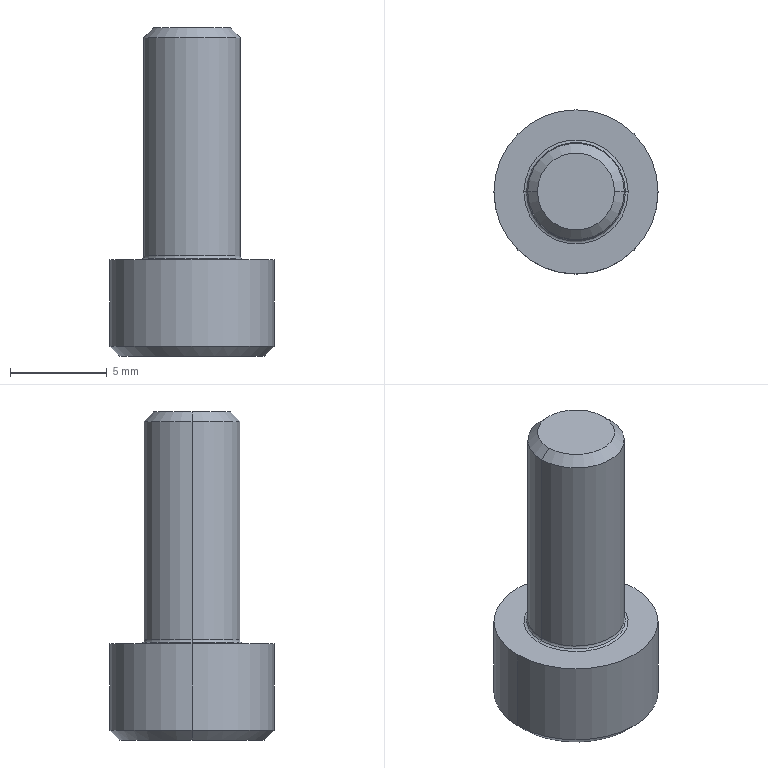Part | Creo | 1 solid | 23 faces | box 8.5 x 8.5 x 17 mm | volume 472.559 mm3 | plane 9 | cone 6 | cylinder 4 | torus 4 | commonest cylinder face diameters 5 x2 8.5 x2
STEP:
#1=CARTESIAN_POINT('',(-86.191,-52.429,-197.5));
#2=VERTEX_POINT('',#1);
#3=CARTESIAN_POINT('',(-87.345,-54.429,-197.5));
#4=VERTEX_POINT('',#3);
#5=CARTESIAN_POINT('',(-86.191,-52.429,-197.5));
#6=CARTESIAN_POINT('',(-86.244,-52.522,-197.469));
#7=CARTESIAN_POINT('',(-86.352,-52.708,-197.413));
#8=CARTESIAN_POINT('',(-86.517,-52.995,-197.352));
#9=CARTESIAN_POINT('',(-86.684,-53.284,-197.32));
#10=CARTESIAN_POINT('',(-86.851,-53.573,-197.32));
#11=CARTESIAN_POINT('',(-87.018,-53.862,-197.352));
#12=CARTESIAN_POINT('',(-87.183,-54.149,-197.413));
#13=CARTESIAN_POINT('',(-87.292,-54.336,-197.469));
#14=CARTESIAN_POINT('',(-87.345,-54.429,-197.5));
#15=B_SPLINE_CURVE_WITH_KNOTS('',3,(#5,#6,#7,#8,#9,#10,#11,#12,#13,#14),.UNSPECIFIED.,.F.,.F.,(4,1,1,1,1,1,1,4),(0.,0.1429,0.2857,0.4286,0.5714,0.7143,0.8571,1.),.UNSPECIFIED.);
#16=EDGE_CURVE('',#2,#4,#15,.T.);
#17=ORIENTED_EDGE('',*,*,#16,.F.);
#18=CARTESIAN_POINT('',(-88.5,-52.429,-196.167));
#19=VERTEX_POINT('',#18);
#20=CARTESIAN_POINT('',(-88.5,-52.429,-196.167));
#21=DIRECTION('',(0.866,0.,-0.5));
#22=VECTOR('',#21,2.667);
#23=LINE('',#20,#22);
#24=EDGE_CURVE('',#19,#2,#23,.T.);
#25=ORIENTED_EDGE('',*,*,#24,.F.);
#26=CARTESIAN_POINT('',(-90.809,-52.429,-197.5));
#27=VERTEX_POINT('',#26);
#28=CARTESIAN_POINT('',(-88.5,-52.429,-196.167));
#29=DIRECTION('',(-0.866,0.,-0.5));
#30=VECTOR('',#29,2.667);
#31=LINE('',#28,#30);
#32=EDGE_CURVE('',#19,#27,#31,.T.);
#33=ORIENTED_EDGE('',*,*,#32,.T.);
#34=CARTESIAN_POINT('',(-89.655,-54.429,-197.5));
#35=VERTEX_POINT('',#34);
#36=CARTESIAN_POINT('',(-89.655,-54.429,-197.5));
#37=CARTESIAN_POINT('',(-89.708,-54.336,-197.469));
#38=CARTESIAN_POINT('',(-89.817,-54.149,-197.413));
#39=CARTESIAN_POINT('',(-89.982,-53.862,-197.352));
#40=CARTESIAN_POINT('',(-90.149,-53.573,-197.32));
#41=CARTESIAN_POINT('',(-90.316,-53.284,-197.32));
#42=CARTESIAN_POINT('',(-90.483,-52.995,-197.352));
#43=CARTESIAN_POINT('',(-90.648,-52.708,-197.413));
#44=CARTESIAN_POINT('',(-90.756,-52.522,-197.469));
#45=CARTESIAN_POINT('',(-90.809,-52.429,-197.5));
#46=B_SPLINE_CURVE_WITH_KNOTS('',3,(#36,#37,#38,#39,#40,#41,#42,#43,#44,#45),.UNSPECIFIED.,.F.,.F.,(4,1,1,1,1,1,1,4),(0.,0.1429,0.2857,0.4286,0.5714,0.7143,0.8571,1.),.UNSPECIFIED.);
#47=EDGE_CURVE('',#35,#27,#46,.T.);
#48=ORIENTED_EDGE('',*,*,#47,.F.);
#49=CARTESIAN_POINT('',(-87.345,-54.429,-197.5));
#50=CARTESIAN_POINT('',(-87.453,-54.429,-197.469));
#51=CARTESIAN_POINT('',(-87.669,-54.429,-197.413));
#52=CARTESIAN_POINT('',(-88.,-54.429,-197.352));
#53=CARTESIAN_POINT('',(-88.334,-54.429,-197.32));
#54=CARTESIAN_POINT('',(-88.668,-54.429,-197.32));
#55=CARTESIAN_POINT('',(-89.002,-54.429,-197.352));
#56=CARTESIAN_POINT('',(-89.332,-54.429,-197.413));
#57=CARTESIAN_POINT('',(-89.548,-54.429,-197.469));
#58=CARTESIAN_POINT('',(-89.655,-54.429,-197.5));
#59=B_SPLINE_CURVE_WITH_KNOTS('',3,(#49,#50,#51,#52,#53,#54,#55,#56,#57,#58),.UNSPECIFIED.,.F.,.F.,(4,1,1,1,1,1,1,4),(0.,0.1429,0.2857,0.4286,0.5714,0.7143,0.8571,1.),.UNSPECIFIED.);
#60=EDGE_CURVE('',#4,#35,#59,.T.);
#61=ORIENTED_EDGE('',*,*,#60,.F.);
#62=EDGE_LOOP('',(#17,#25,#33,#48,#61));
#63=FACE_OUTER_BOUND('',#62,.F.);
#64=CARTESIAN_POINT('',(-88.5,-52.429,-196.847));
#65=DIRECTION('',(0.,0.,-1.));
#66=DIRECTION('',(1.,0.,0.));
#67=AXIS2_PLACEMENT_3D('',#64,#65,#66);
#68=CONICAL_SURFACE('',#67,1.178,60.);
#69=ADVANCED_FACE('',(#63),#68,.F.);
#70=CARTESIAN_POINT('',(-87.345,-54.429,-200.));
#71=VERTEX_POINT('',#70);
#72=CARTESIAN_POINT('',(-86.191,-52.429,-200.));
#73=VERTEX_POINT('',#72);
#74=CARTESIAN_POINT('',(-87.345,-54.429,-200.));
#75=DIRECTION('',(0.5,0.866,0.));
#76=VECTOR('',#75,2.309);
#77=LINE('',#74,#76);
#78=EDGE_CURVE('',#71,#73,#77,.T.);
#79=ORIENTED_EDGE('',*,*,#78,.T.);
#80=CARTESIAN_POINT('',(-86.191,-52.429,-197.5));
#81=DIRECTION('',(0.,0.,-1.));
#82=VECTOR('',#81,2.5);
#83=LINE('',#80,#82);
#84=EDGE_CURVE('',#2,#73,#83,.T.);
#85=ORIENTED_EDGE('',*,*,#84,.F.);
#86=ORIENTED_EDGE('',*,*,#16,.T.);
#87=CARTESIAN_POINT('',(-87.345,-54.429,-197.5));
#88=DIRECTION('',(0.,0.,-1.));
#89=VECTOR('',#88,2.5);
#90=LINE('',#87,#89);
#91=EDGE_CURVE('',#4,#71,#90,.T.);
#92=ORIENTED_EDGE('',*,*,#91,.T.);
#93=EDGE_LOOP('',(#79,#85,#86,#92));
#94=FACE_OUTER_BOUND('',#93,.F.);
#95=CARTESIAN_POINT('',(-87.345,-54.429,-197.5));
#96=DIRECTION('',(-0.866,0.5,0.));
#97=DIRECTION('',(-0.5,-0.866,0.));
#98=AXIS2_PLACEMENT_3D('',#95,#96,#97);
#99=PLANE('',#98);
#100=ADVANCED_FACE('',(#94),#99,.T.);
#101=CARTESIAN_POINT('',(-92.25,-52.429,-200.));
#102=VERTEX_POINT('',#101);
#103=CARTESIAN_POINT('',(-84.75,-52.429,-200.));
#104=VERTEX_POINT('',#103);
#105=CARTESIAN_POINT('',(-88.5,-52.429,-200.));
#106=DIRECTION('',(0.,0.,-1.));
#107=DIRECTION('',(-1.,0.,0.));
#108=AXIS2_PLACEMENT_3D('',#105,#106,#107);
#109=CIRCLE('',#108,3.75);
#110=EDGE_CURVE('',#102,#104,#109,.T.);
#111=ORIENTED_EDGE('',*,*,#110,.F.);
#112=CARTESIAN_POINT('',(-88.5,-52.429,-200.));
#113=DIRECTION('',(0.,0.,-1.));
#114=DIRECTION('',(1.,0.,0.));
#115=AXIS2_PLACEMENT_3D('',#112,#113,#114);
#116=CIRCLE('',#115,3.75);
#117=EDGE_CURVE('',#104,#102,#116,.T.);
#118=ORIENTED_EDGE('',*,*,#117,.F.);
#119=EDGE_LOOP('',(#111,#118));
#120=FACE_OUTER_BOUND('',#119,.F.);
#121=CARTESIAN_POINT('',(-90.809,-52.429,-200.));
#122=VERTEX_POINT('',#121);
#123=CARTESIAN_POINT('',(-89.655,-54.429,-200.));
#124=VERTEX_POINT('',#123);
#125=CARTESIAN_POINT('',(-90.809,-52.429,-200.));
#126=DIRECTION('',(0.5,-0.866,0.));
#127=VECTOR('',#126,2.309);
#128=LINE('',#125,#127);
#129=EDGE_CURVE('',#122,#124,#128,.T.);
#130=ORIENTED_EDGE('',*,*,#129,.F.);
#131=CARTESIAN_POINT('',(-89.655,-50.429,-200.));
#132=VERTEX_POINT('',#131);
#133=CARTESIAN_POINT('',(-89.655,-50.429,-200.));
#134=DIRECTION('',(-0.5,-0.866,0.));
#135=VECTOR('',#134,2.309);
#136=LINE('',#133,#135);
#137=EDGE_CURVE('',#132,#122,#136,.T.);
#138=ORIENTED_EDGE('',*,*,#137,.F.);
#139=CARTESIAN_POINT('',(-87.345,-50.429,-200.));
#140=VERTEX_POINT('',#139);
#141=CARTESIAN_POINT('',(-89.655,-50.429,-200.));
#142=DIRECTION('',(1.,0.,0.));
#143=VECTOR('',#142,2.309);
#144=LINE('',#141,#143);
#145=EDGE_CURVE('',#132,#140,#144,.T.);
#146=ORIENTED_EDGE('',*,*,#145,.T.);
#147=CARTESIAN_POINT('',(-86.191,-52.429,-200.));
#148=DIRECTION('',(-0.5,0.866,0.));
#149=VECTOR('',#148,2.309);
#150=LINE('',#147,#149);
#151=EDGE_CURVE('',#73,#140,#150,.T.);
#152=ORIENTED_EDGE('',*,*,#151,.F.);
#153=ORIENTED_EDGE('',*,*,#78,.F.);
#154=CARTESIAN_POINT('',(-87.345,-54.429,-200.));
#155=DIRECTION('',(-1.,0.,0.));
#156=VECTOR('',#155,2.309);
#157=LINE('',#154,#156);
#158=EDGE_CURVE('',#71,#124,#157,.T.);
#159=ORIENTED_EDGE('',*,*,#158,.T.);
#160=EDGE_LOOP('',(#130,#138,#146,#152,#153,#159));
#161=FACE_BOUND('',#160,.F.);
#162=CARTESIAN_POINT('',(-88.5,-52.429,-200.));
#163=DIRECTION('',(0.,0.,-1.));
#164=DIRECTION('',(1.,0.,0.));
#165=AXIS2_PLACEMENT_3D('',#162,#163,#164);
#166=PLANE('',#165);
#167=ADVANCED_FACE('',(#120,#161),#166,.T.);
#168=CARTESIAN_POINT('',(-92.75,-52.429,-199.5));
#169=VERTEX_POINT('',#168);
#170=CARTESIAN_POINT('',(-84.25,-52.429,-199.5));
#171=VERTEX_POINT('',#170);
#172=CARTESIAN_POINT('',(-88.5,-52.429,-199.5));
#173=DIRECTION('',(0.,0.,-1.));
#174=DIRECTION('',(-1.,0.,0.));
#175=AXIS2_PLACEMENT_3D('',#172,#173,#174);
#176=CIRCLE('',#175,4.25);
#177=EDGE_CURVE('',#169,#171,#176,.T.);
#178=ORIENTED_EDGE('',*,*,#177,.F.);
#179=CARTESIAN_POINT('',(-92.25,-52.429,-200.));
#180=DIRECTION('',(-0.7071,0.,0.7071));
#181=VECTOR('',#180,0.7071);
#182=LINE('',#179,#181);
#183=EDGE_CURVE('',#102,#169,#182,.T.);
#184=ORIENTED_EDGE('',*,*,#183,.F.);
#185=ORIENTED_EDGE('',*,*,#110,.T.);
#186=CARTESIAN_POINT('',(-84.75,-52.429,-200.));
#187=DIRECTION('',(0.7071,0.,0.7071));
#188=VECTOR('',#187,0.7071);
#189=LINE('',#186,#188);
#190=EDGE_CURVE('',#104,#171,#189,.T.);
#191=ORIENTED_EDGE('',*,*,#190,.T.);
#192=EDGE_LOOP('',(#178,#184,#185,#191));
#193=FACE_OUTER_BOUND('',#192,.F.);
#194=CARTESIAN_POINT('',(-88.5,-52.429,-199.75));
#195=DIRECTION('',(0.,0.,1.));
#196=DIRECTION('',(-1.,0.,0.));
#197=AXIS2_PLACEMENT_3D('',#194,#195,#196);
#198=CONICAL_SURFACE('',#197,4.,45.);
#199=ADVANCED_FACE('',(#193),#198,.T.);
#200=ORIENTED_EDGE('',*,*,#177,.T.);
#201=CARTESIAN_POINT('',(-84.25,-52.429,-195.));
#202=VERTEX_POINT('',#201);
#203=CARTESIAN_POINT('',(-84.25,-52.429,-195.));
#204=DIRECTION('',(0.,0.,-1.));
#205=VECTOR('',#204,4.5);
#206=LINE('',#203,#205);
#207=EDGE_CURVE('',#202,#171,#206,.T.);
#208=ORIENTED_EDGE('',*,*,#207,.F.);
#209=CARTESIAN_POINT('',(-92.75,-52.429,-195.));
#210=VERTEX_POINT('',#209);
#211=CARTESIAN_POINT('',(-88.5,-52.429,-195.));
#212=DIRECTION('',(0.,0.,1.));
#213=DIRECTION('',(1.,0.,0.));
#214=AXIS2_PLACEMENT_3D('',#211,#212,#213);
#215=CIRCLE('',#214,4.25);
#216=EDGE_CURVE('',#202,#210,#215,.T.);
#217=ORIENTED_EDGE('',*,*,#216,.T.);
#218=CARTESIAN_POINT('',(-92.75,-52.429,-195.));
#219=DIRECTION('',(0.,0.,-1.));
#220=VECTOR('',#219,4.5);
#221=LINE('',#218,#220);
#222=EDGE_CURVE('',#210,#169,#221,.T.);
#223=ORIENTED_EDGE('',*,*,#222,.T.);
#224=EDGE_LOOP('',(#200,#208,#217,#223));
#225=FACE_OUTER_BOUND('',#224,.F.);
#226=CARTESIAN_POINT('',(-88.5,-52.429,-195.));
#227=DIRECTION('',(0.,0.,-1.));
#228=DIRECTION('',(1.,0.,0.));
#229=AXIS2_PLACEMENT_3D('',#226,#227,#228);
#230=CYLINDRICAL_SURFACE('',#229,4.25);
#231=ADVANCED_FACE('',(#225),#230,.T.);
#232=CARTESIAN_POINT('',(-88.5,-52.429,-199.5));
#233=DIRECTION('',(0.,0.,-1.));
#234=DIRECTION('',(1.,0.,0.));
#235=AXIS2_PLACEMENT_3D('',#232,#233,#234);
#236=CIRCLE('',#235,4.25);
#237=EDGE_CURVE('',#171,#169,#236,.T.);
#238=ORIENTED_EDGE('',*,*,#237,.T.);
#239=ORIENTED_EDGE('',*,*,#222,.F.);
#240=CARTESIAN_POINT('',(-88.5,-52.429,-195.));
#241=DIRECTION('',(0.,0.,1.));
#242=DIRECTION('',(-1.,0.,0.));
#243=AXIS2_PLACEMENT_3D('',#240,#241,#242);
#244=CIRCLE('',#243,4.25);
#245=EDGE_CURVE('',#210,#202,#244,.T.);
#246=ORIENTED_EDGE('',*,*,#245,.T.);
#247=ORIENTED_EDGE('',*,*,#207,.T.);
#248=EDGE_LOOP('',(#238,#239,#246,#247));
#249=FACE_OUTER_BOUND('',#248,.F.);
#250=CARTESIAN_POINT('',(-88.5,-52.429,-195.));
#251=DIRECTION('',(0.,0.,-1.));
#252=DIRECTION('',(1.,0.,0.));
#253=AXIS2_PLACEMENT_3D('',#250,#251,#252);
#254=CYLINDRICAL_SURFACE('',#253,4.25);
#255=ADVANCED_FACE('',(#249),#254,.T.);
#256=ORIENTED_EDGE('',*,*,#237,.F.);
#257=ORIENTED_EDGE('',*,*,#190,.F.);
#258=ORIENTED_EDGE('',*,*,#117,.T.);
#259=ORIENTED_EDGE('',*,*,#183,.T.);
#260=EDGE_LOOP('',(#256,#257,#258,#259));
#261=FACE_OUTER_BOUND('',#260,.F.);
#262=CARTESIAN_POINT('',(-88.5,-52.429,-199.75));
#263=DIRECTION('',(0.,0.,1.));
#264=DIRECTION('',(-1.,0.,0.));
#265=AXIS2_PLACEMENT_3D('',#262,#263,#264);
#266=CONICAL_SURFACE('',#265,4.,45.);
#267=ADVANCED_FACE('',(#261),#266,.T.);
#268=ORIENTED_EDGE('',*,*,#245,.F.);
#269=ORIENTED_EDGE('',*,*,#216,.F.);
#270=EDGE_LOOP('',(#268,#269));
#271=FACE_OUTER_BOUND('',#270,.F.);
#272=CARTESIAN_POINT('',(-91.2,-52.429,-195.));
#273=VERTEX_POINT('',#272);
#274=CARTESIAN_POINT('',(-85.8,-52.429,-195.));
#275=VERTEX_POINT('',#274);
#276=CARTESIAN_POINT('',(-88.5,-52.429,-195.));
#277=DIRECTION('',(0.,0.,-1.));
#278=DIRECTION('',(-1.,0.,0.));
#279=AXIS2_PLACEMENT_3D('',#276,#277,#278);
#280=CIRCLE('',#279,2.7);
#281=EDGE_CURVE('',#273,#275,#280,.T.);
#282=ORIENTED_EDGE('',*,*,#281,.F.);
#283=CARTESIAN_POINT('',(-88.5,-52.429,-195.));
#284=DIRECTION('',(0.,0.,-1.));
#285=DIRECTION('',(1.,0.,0.));
#286=AXIS2_PLACEMENT_3D('',#283,#284,#285);
#287=CIRCLE('',#286,2.7);
#288=EDGE_CURVE('',#275,#273,#287,.T.);
#289=ORIENTED_EDGE('',*,*,#288,.F.);
#290=EDGE_LOOP('',(#282,#289));
#291=FACE_BOUND('',#290,.F.);
#292=CARTESIAN_POINT('',(-88.5,-52.429,-195.));
#293=DIRECTION('',(0.,0.,-1.));
#294=DIRECTION('',(1.,0.,0.));
#295=AXIS2_PLACEMENT_3D('',#292,#293,#294);
#296=PLANE('',#295);
#297=ADVANCED_FACE('',(#271,#291),#296,.F.);
#298=ORIENTED_EDGE('',*,*,#281,.T.);
#299=CARTESIAN_POINT('',(-85.941,-52.429,-194.941));
#300=VERTEX_POINT('',#299);
#301=CARTESIAN_POINT('',(-85.8,-52.429,-194.8));
#302=DIRECTION('',(0.,1.,0.));
#303=DIRECTION('',(0.,0.,-1.));
#304=AXIS2_PLACEMENT_3D('',#301,#302,#303);
#305=CIRCLE('',#304,0.2);
#306=EDGE_CURVE('',#275,#300,#305,.T.);
#307=ORIENTED_EDGE('',*,*,#306,.T.);
#308=CARTESIAN_POINT('',(-91.059,-52.429,-194.941));
#309=VERTEX_POINT('',#308);
#310=CARTESIAN_POINT('',(-88.5,-52.429,-194.941));
#311=DIRECTION('',(0.,0.,-1.));
#312=DIRECTION('',(-1.,0.,0.));
#313=AXIS2_PLACEMENT_3D('',#310,#311,#312);
#314=CIRCLE('',#313,2.559);
#315=EDGE_CURVE('',#309,#300,#314,.T.);
#316=ORIENTED_EDGE('',*,*,#315,.F.);
#317=CARTESIAN_POINT('',(-91.2,-52.429,-194.8));
#318=DIRECTION('',(0.,-1.,0.));
#319=DIRECTION('',(0.,0.,-1.));
#320=AXIS2_PLACEMENT_3D('',#317,#318,#319);
#321=CIRCLE('',#320,0.2);
#322=EDGE_CURVE('',#273,#309,#321,.T.);
#323=ORIENTED_EDGE('',*,*,#322,.F.);
#324=EDGE_LOOP('',(#298,#307,#316,#323));
#325=FACE_OUTER_BOUND('',#324,.F.);
#326=CARTESIAN_POINT('',(-88.5,-52.429,-194.8));
#327=DIRECTION('',(0.,0.,-1.));
#328=DIRECTION('',(1.,0.,0.));
#329=AXIS2_PLACEMENT_3D('',#326,#327,#328);
#330=TOROIDAL_SURFACE('',#329,2.7,0.2);
#331=ADVANCED_FACE('',(#325),#330,.F.);
#332=ORIENTED_EDGE('',*,*,#288,.T.);
#333=ORIENTED_EDGE('',*,*,#322,.T.);
#334=CARTESIAN_POINT('',(-88.5,-52.429,-194.941));
#335=DIRECTION('',(0.,0.,-1.));
#336=DIRECTION('',(1.,0.,0.));
#337=AXIS2_PLACEMENT_3D('',#334,#335,#336);
#338=CIRCLE('',#337,2.559);
#339=EDGE_CURVE('',#300,#309,#338,.T.);
#340=ORIENTED_EDGE('',*,*,#339,.F.);
#341=ORIENTED_EDGE('',*,*,#306,.F.);
#342=EDGE_LOOP('',(#332,#333,#340,#341));
#343=FACE_OUTER_BOUND('',#342,.F.);
#344=CARTESIAN_POINT('',(-88.5,-52.429,-194.8));
#345=DIRECTION('',(0.,0.,-1.));
#346=DIRECTION('',(1.,0.,0.));
#347=AXIS2_PLACEMENT_3D('',#344,#345,#346);
#348=TOROIDAL_SURFACE('',#347,2.7,0.2);
#349=ADVANCED_FACE('',(#343),#348,.F.);
#350=CARTESIAN_POINT('',(-86.,-52.429,-194.8));
#351=VERTEX_POINT('',#350);
#352=CARTESIAN_POINT('',(-91.,-52.429,-194.8));
#353=VERTEX_POINT('',#352);
#354=CARTESIAN_POINT('',(-88.5,-52.429,-194.8));
#355=DIRECTION('',(0.,0.,-1.));
#356=DIRECTION('',(1.,0.,0.));
#357=AXIS2_PLACEMENT_3D('',#354,#355,#356);
#358=CIRCLE('',#357,2.5);
#359=EDGE_CURVE('',#351,#353,#358,.T.);
#360=ORIENTED_EDGE('',*,*,#359,.F.);
#361=CARTESIAN_POINT('',(-85.8,-52.429,-194.8));
#362=DIRECTION('',(0.,1.,0.));
#363=DIRECTION('',(-0.7071,0.,-0.7071));
#364=AXIS2_PLACEMENT_3D('',#361,#362,#363);
#365=CIRCLE('',#364,0.2);
#366=EDGE_CURVE('',#300,#351,#365,.T.);
#367=ORIENTED_EDGE('',*,*,#366,.F.);
#368=ORIENTED_EDGE('',*,*,#339,.T.);
#369=CARTESIAN_POINT('',(-91.2,-52.429,-194.8));
#370=DIRECTION('',(0.,-1.,0.));
#371=DIRECTION('',(0.7071,0.,-0.7071));
#372=AXIS2_PLACEMENT_3D('',#369,#370,#371);
#373=CIRCLE('',#372,0.2);
#374=EDGE_CURVE('',#309,#353,#373,.T.);
#375=ORIENTED_EDGE('',*,*,#374,.T.);
#376=EDGE_LOOP('',(#360,#367,#368,#375));
#377=FACE_OUTER_BOUND('',#376,.F.);
#378=CARTESIAN_POINT('',(-88.5,-52.429,-194.8));
#379=DIRECTION('',(0.,0.,-1.));
#380=DIRECTION('',(1.,0.,0.));
#381=AXIS2_PLACEMENT_3D('',#378,#379,#380);
#382=TOROIDAL_SURFACE('',#381,2.7,0.2);
#383=ADVANCED_FACE('',(#377),#382,.F.);
#384=CARTESIAN_POINT('',(-91.,-52.429,-183.5));
#385=VERTEX_POINT('',#384);
#386=CARTESIAN_POINT('',(-86.,-52.429,-183.5));
#387=VERTEX_POINT('',#386);
#388=CARTESIAN_POINT('',(-88.5,-52.429,-183.5));
#389=DIRECTION('',(0.,0.,1.));
#390=DIRECTION('',(-1.,0.,0.));
#391=AXIS2_PLACEMENT_3D('',#388,#389,#390);
#392=CIRCLE('',#391,2.5);
#393=EDGE_CURVE('',#385,#387,#392,.T.);
#394=ORIENTED_EDGE('',*,*,#393,.T.);
#395=CARTESIAN_POINT('',(-86.,-52.429,-183.5));
#396=DIRECTION('',(0.,0.,-1.));
#397=VECTOR('',#396,11.3);
#398=LINE('',#395,#397);
#399=EDGE_CURVE('',#387,#351,#398,.T.);
#400=ORIENTED_EDGE('',*,*,#399,.T.);
#401=ORIENTED_EDGE('',*,*,#359,.T.);
#402=CARTESIAN_POINT('',(-91.,-52.429,-183.5));
#403=DIRECTION('',(0.,0.,-1.));
#404=VECTOR('',#403,11.3);
#405=LINE('',#402,#404);
#406=EDGE_CURVE('',#385,#353,#405,.T.);
#407=ORIENTED_EDGE('',*,*,#406,.F.);
#408=EDGE_LOOP('',(#394,#400,#401,#407));
#409=FACE_OUTER_BOUND('',#408,.F.);
#410=CARTESIAN_POINT('',(-88.5,-52.429,-183.));
#411=DIRECTION('',(0.,0.,-1.));
#412=DIRECTION('',(1.,0.,0.));
#413=AXIS2_PLACEMENT_3D('',#410,#411,#412);
#414=CYLINDRICAL_SURFACE('',#413,2.5);
#415=ADVANCED_FACE('',(#409),#414,.T.);
#416=CARTESIAN_POINT('',(-90.5,-52.429,-183.));
#417=VERTEX_POINT('',#416);
#418=CARTESIAN_POINT('',(-86.5,-52.429,-183.));
#419=VERTEX_POINT('',#418);
#420=CARTESIAN_POINT('',(-88.5,-52.429,-183.));
#421=DIRECTION('',(0.,0.,1.));
#422=DIRECTION('',(-1.,0.,0.));
#423=AXIS2_PLACEMENT_3D('',#420,#421,#422);
#424=CIRCLE('',#423,2.);
#425=EDGE_CURVE('',#417,#419,#424,.T.);
#426=ORIENTED_EDGE('',*,*,#425,.T.);
#427=CARTESIAN_POINT('',(-86.5,-52.429,-183.));
#428=DIRECTION('',(0.7071,0.,-0.7071));
#429=VECTOR('',#428,0.7071);
#430=LINE('',#427,#429);
#431=EDGE_CURVE('',#419,#387,#430,.T.);
#432=ORIENTED_EDGE('',*,*,#431,.T.);
#433=ORIENTED_EDGE('',*,*,#393,.F.);
#434=CARTESIAN_POINT('',(-90.5,-52.429,-183.));
#435=DIRECTION('',(-0.7071,0.,-0.7071));
#436=VECTOR('',#435,0.7071);
#437=LINE('',#434,#436);
#438=EDGE_CURVE('',#417,#385,#437,.T.);
#439=ORIENTED_EDGE('',*,*,#438,.F.);
#440=EDGE_LOOP('',(#426,#432,#433,#439));
#441=FACE_OUTER_BOUND('',#440,.F.);
#442=CARTESIAN_POINT('',(-88.5,-52.429,-183.25));
#443=DIRECTION('',(0.,0.,-1.));
#444=DIRECTION('',(1.,0.,0.));
#445=AXIS2_PLACEMENT_3D('',#442,#443,#444);
#446=CONICAL_SURFACE('',#445,2.25,45.);
#447=ADVANCED_FACE('',(#441),#446,.T.);
#448=ORIENTED_EDGE('',*,*,#425,.F.);
#449=CARTESIAN_POINT('',(-88.5,-52.429,-183.));
#450=DIRECTION('',(0.,0.,1.));
#451=DIRECTION('',(1.,0.,0.));
#452=AXIS2_PLACEMENT_3D('',#449,#450,#451);
#453=CIRCLE('',#452,2.);
#454=EDGE_CURVE('',#419,#417,#453,.T.);
#455=ORIENTED_EDGE('',*,*,#454,.F.);
#456=EDGE_LOOP('',(#448,#455));
#457=FACE_OUTER_BOUND('',#456,.F.);
#458=CARTESIAN_POINT('',(-88.5,-52.429,-183.));
#459=DIRECTION('',(0.,0.,-1.));
#460=DIRECTION('',(1.,0.,0.));
#461=AXIS2_PLACEMENT_3D('',#458,#459,#460);
#462=PLANE('',#461);
#463=ADVANCED_FACE('',(#457),#462,.F.);
#464=ORIENTED_EDGE('',*,*,#454,.T.);
#465=ORIENTED_EDGE('',*,*,#438,.T.);
#466=CARTESIAN_POINT('',(-88.5,-52.429,-183.5));
#467=DIRECTION('',(0.,0.,1.));
#468=DIRECTION('',(1.,0.,0.));
#469=AXIS2_PLACEMENT_3D('',#466,#467,#468);
#470=CIRCLE('',#469,2.5);
#471=EDGE_CURVE('',#387,#385,#470,.T.);
#472=ORIENTED_EDGE('',*,*,#471,.F.);
#473=ORIENTED_EDGE('',*,*,#431,.F.);
#474=EDGE_LOOP('',(#464,#465,#472,#473));
#475=FACE_OUTER_BOUND('',#474,.F.);
#476=CARTESIAN_POINT('',(-88.5,-52.429,-183.25));
#477=DIRECTION('',(0.,0.,-1.));
#478=DIRECTION('',(1.,0.,0.));
#479=AXIS2_PLACEMENT_3D('',#476,#477,#478);
#480=CONICAL_SURFACE('',#479,2.25,45.);
#481=ADVANCED_FACE('',(#475),#480,.T.);
#482=ORIENTED_EDGE('',*,*,#471,.T.);
#483=ORIENTED_EDGE('',*,*,#406,.T.);
#484=CARTESIAN_POINT('',(-88.5,-52.429,-194.8));
#485=DIRECTION('',(0.,0.,-1.));
#486=DIRECTION('',(-1.,0.,0.));
#487=AXIS2_PLACEMENT_3D('',#484,#485,#486);
#488=CIRCLE('',#487,2.5);
#489=EDGE_CURVE('',#353,#351,#488,.T.);
#490=ORIENTED_EDGE('',*,*,#489,.T.);
#491=ORIENTED_EDGE('',*,*,#399,.F.);
#492=EDGE_LOOP('',(#482,#483,#490,#491));
#493=FACE_OUTER_BOUND('',#492,.F.);
#494=CARTESIAN_POINT('',(-88.5,-52.429,-183.));
#495=DIRECTION('',(0.,0.,-1.));
#496=DIRECTION('',(1.,0.,0.));
#497=AXIS2_PLACEMENT_3D('',#494,#495,#496);
#498=CYLINDRICAL_SURFACE('',#497,2.5);
#499=ADVANCED_FACE('',(#493),#498,.T.);
#500=ORIENTED_EDGE('',*,*,#489,.F.);
#501=ORIENTED_EDGE('',*,*,#374,.F.);
#502=ORIENTED_EDGE('',*,*,#315,.T.);
#503=ORIENTED_EDGE('',*,*,#366,.T.);
#504=EDGE_LOOP('',(#500,#501,#502,#503));
#505=FACE_OUTER_BOUND('',#504,.F.);
#506=CARTESIAN_POINT('',(-88.5,-52.429,-194.8));
#507=DIRECTION('',(0.,0.,-1.));
#508=DIRECTION('',(1.,0.,0.));
#509=AXIS2_PLACEMENT_3D('',#506,#507,#508);
#510=TOROIDAL_SURFACE('',#509,2.7,0.2);
#511=ADVANCED_FACE('',(#505),#510,.F.);
#512=ORIENTED_EDGE('',*,*,#129,.T.);
#513=CARTESIAN_POINT('',(-89.655,-54.429,-197.5));
#514=DIRECTION('',(0.,0.,-1.));
#515=VECTOR('',#514,2.5);
#516=LINE('',#513,#515);
#517=EDGE_CURVE('',#35,#124,#516,.T.);
#518=ORIENTED_EDGE('',*,*,#517,.F.);
#519=ORIENTED_EDGE('',*,*,#47,.T.);
#520=CARTESIAN_POINT('',(-90.809,-52.429,-197.5));
#521=DIRECTION('',(0.,0.,-1.));
#522=VECTOR('',#521,2.5);
#523=LINE('',#520,#522);
#524=EDGE_CURVE('',#27,#122,#523,.T.);
#525=ORIENTED_EDGE('',*,*,#524,.T.);
#526=EDGE_LOOP('',(#512,#518,#519,#525));
#527=FACE_OUTER_BOUND('',#526,.F.);
#528=CARTESIAN_POINT('',(-90.809,-52.429,-197.5));
#529=DIRECTION('',(0.866,0.5,0.));
#530=DIRECTION('',(-0.5,0.866,0.));
#531=AXIS2_PLACEMENT_3D('',#528,#529,#530);
#532=PLANE('',#531);
#533=ADVANCED_FACE('',(#527),#532,.T.);
#534=ORIENTED_EDGE('',*,*,#158,.F.);
#535=ORIENTED_EDGE('',*,*,#91,.F.);
#536=ORIENTED_EDGE('',*,*,#60,.T.);
#537=ORIENTED_EDGE('',*,*,#517,.T.);
#538=EDGE_LOOP('',(#534,#535,#536,#537));
#539=FACE_OUTER_BOUND('',#538,.F.);
#540=CARTESIAN_POINT('',(-89.655,-54.429,-197.5));
#541=DIRECTION('',(0.,1.,0.));
#542=DIRECTION('',(0.,0.,1.));
#543=AXIS2_PLACEMENT_3D('',#540,#541,#542);
#544=PLANE('',#543);
#545=ADVANCED_FACE('',(#539),#544,.T.);
#546=ORIENTED_EDGE('',*,*,#137,.T.);
#547=ORIENTED_EDGE('',*,*,#524,.F.);
#548=CARTESIAN_POINT('',(-89.655,-50.429,-197.5));
#549=VERTEX_POINT('',#548);
#550=CARTESIAN_POINT('',(-90.809,-52.429,-197.5));
#551=CARTESIAN_POINT('',(-90.756,-52.336,-197.469));
#552=CARTESIAN_POINT('',(-90.648,-52.149,-197.413));
#553=CARTESIAN_POINT('',(-90.482,-51.862,-197.352));
#554=CARTESIAN_POINT('',(-90.315,-51.573,-197.32));
#555=CARTESIAN_POINT('',(-90.148,-51.284,-197.32));
#556=CARTESIAN_POINT('',(-89.981,-50.995,-197.352));
#557=CARTESIAN_POINT('',(-89.816,-50.708,-197.413));
#558=CARTESIAN_POINT('',(-89.708,-50.522,-197.469));
#559=CARTESIAN_POINT('',(-89.655,-50.429,-197.5));
#560=B_SPLINE_CURVE_WITH_KNOTS('',3,(#550,#551,#552,#553,#554,#555,#556,#557,#558,#559),.UNSPECIFIED.,.F.,.F.,(4,1,1,1,1,1,1,4),(0.,0.1429,0.2857,0.4286,0.5714,0.7143,0.8571,1.),.UNSPECIFIED.);
#561=EDGE_CURVE('',#27,#549,#560,.T.);
#562=ORIENTED_EDGE('',*,*,#561,.T.);
#563=CARTESIAN_POINT('',(-89.655,-50.429,-197.5));
#564=DIRECTION('',(0.,0.,-1.));
#565=VECTOR('',#564,2.5);
#566=LINE('',#563,#565);
#567=EDGE_CURVE('',#549,#132,#566,.T.);
#568=ORIENTED_EDGE('',*,*,#567,.T.);
#569=EDGE_LOOP('',(#546,#547,#562,#568));
#570=FACE_OUTER_BOUND('',#569,.F.);
#571=CARTESIAN_POINT('',(-89.655,-50.429,-197.5));
#572=DIRECTION('',(0.866,-0.5,0.));
#573=DIRECTION('',(0.5,0.866,0.));
#574=AXIS2_PLACEMENT_3D('',#571,#572,#573);
#575=PLANE('',#574);
#576=ADVANCED_FACE('',(#570),#575,.T.);
#577=ORIENTED_EDGE('',*,*,#561,.F.);
#578=ORIENTED_EDGE('',*,*,#32,.F.);
#579=ORIENTED_EDGE('',*,*,#24,.T.);
#580=CARTESIAN_POINT('',(-87.345,-50.429,-197.5));
#581=VERTEX_POINT('',#580);
#582=CARTESIAN_POINT('',(-87.345,-50.429,-197.5));
#583=CARTESIAN_POINT('',(-87.292,-50.522,-197.469));
#584=CARTESIAN_POINT('',(-87.183,-50.71,-197.413));
#585=CARTESIAN_POINT('',(-87.018,-50.996,-197.352));
#586=CARTESIAN_POINT('',(-86.851,-51.285,-197.32));
#587=CARTESIAN_POINT('',(-86.684,-51.575,-197.32));
#588=CARTESIAN_POINT('',(-86.517,-51.864,-197.352));
#589=CARTESIAN_POINT('',(-86.352,-52.15,-197.413));
#590=CARTESIAN_POINT('',(-86.244,-52.337,-197.469));
#591=CARTESIAN_POINT('',(-86.191,-52.429,-197.5));
#592=B_SPLINE_CURVE_WITH_KNOTS('',3,(#582,#583,#584,#585,#586,#587,#588,#589,#590,#591),.UNSPECIFIED.,.F.,.F.,(4,1,1,1,1,1,1,4),(0.,0.1429,0.2857,0.4286,0.5714,0.7143,0.8571,1.),.UNSPECIFIED.);
#593=EDGE_CURVE('',#581,#2,#592,.T.);
#594=ORIENTED_EDGE('',*,*,#593,.F.);
#595=CARTESIAN_POINT('',(-89.655,-50.429,-197.5));
#596=CARTESIAN_POINT('',(-89.548,-50.429,-197.469));
#597=CARTESIAN_POINT('',(-89.332,-50.429,-197.413));
#598=CARTESIAN_POINT('',(-89.002,-50.429,-197.352));
#599=CARTESIAN_POINT('',(-88.668,-50.429,-197.32));
#600=CARTESIAN_POINT('',(-88.334,-50.429,-197.32));
#601=CARTESIAN_POINT('',(-88.,-50.429,-197.352));
#602=CARTESIAN_POINT('',(-87.669,-50.429,-197.413));
#603=CARTESIAN_POINT('',(-87.453,-50.429,-197.469));
#604=CARTESIAN_POINT('',(-87.345,-50.429,-197.5));
#605=B_SPLINE_CURVE_WITH_KNOTS('',3,(#595,#596,#597,#598,#599,#600,#601,#602,#603,#604),.UNSPECIFIED.,.F.,.F.,(4,1,1,1,1,1,1,4),(0.,0.1429,0.2857,0.4286,0.5714,0.7143,0.8571,1.),.UNSPECIFIED.);
#606=EDGE_CURVE('',#549,#581,#605,.T.);
#607=ORIENTED_EDGE('',*,*,#606,.F.);
#608=EDGE_LOOP('',(#577,#578,#579,#594,#607));
#609=FACE_OUTER_BOUND('',#608,.F.);
#610=CARTESIAN_POINT('',(-88.5,-52.429,-196.847));
#611=DIRECTION('',(0.,0.,-1.));
#612=DIRECTION('',(1.,0.,0.));
#613=AXIS2_PLACEMENT_3D('',#610,#611,#612);
#614=CONICAL_SURFACE('',#613,1.178,60.);
#615=ADVANCED_FACE('',(#609),#614,.F.);
#616=ORIENTED_EDGE('',*,*,#151,.T.);
#617=CARTESIAN_POINT('',(-87.345,-50.429,-197.5));
#618=DIRECTION('',(0.,0.,-1.));
#619=VECTOR('',#618,2.5);
#620=LINE('',#617,#619);
#621=EDGE_CURVE('',#581,#140,#620,.T.);
#622=ORIENTED_EDGE('',*,*,#621,.F.);
#623=ORIENTED_EDGE('',*,*,#593,.T.);
#624=ORIENTED_EDGE('',*,*,#84,.T.);
#625=EDGE_LOOP('',(#616,#622,#623,#624));
#626=FACE_OUTER_BOUND('',#625,.F.);
#627=CARTESIAN_POINT('',(-86.191,-52.429,-197.5));
#628=DIRECTION('',(-0.866,-0.5,0.));
#629=DIRECTION('',(0.5,-0.866,0.));
#630=AXIS2_PLACEMENT_3D('',#627,#628,#629);
#631=PLANE('',#630);
#632=ADVANCED_FACE('',(#626),#631,.T.);
#633=ORIENTED_EDGE('',*,*,#145,.F.);
#634=ORIENTED_EDGE('',*,*,#567,.F.);
#635=ORIENTED_EDGE('',*,*,#606,.T.);
#636=ORIENTED_EDGE('',*,*,#621,.T.);
#637=EDGE_LOOP('',(#633,#634,#635,#636));
#638=FACE_OUTER_BOUND('',#637,.F.);
#639=CARTESIAN_POINT('',(-87.345,-50.429,-197.5));
#640=DIRECTION('',(0.,-1.,0.));
#641=DIRECTION('',(0.,0.,-1.));
#642=AXIS2_PLACEMENT_3D('',#639,#640,#641);
#643=PLANE('',#642);
#644=ADVANCED_FACE('',(#638),#643,.T.);
#645=CLOSED_SHELL('',(#69,#100,#167,#199,#231,#255,#267,#297,#331,#349,#383,#415,#447,#463,#481,#499,#511,#533,#545,#576,#615,#632,#644));
#646=MANIFOLD_SOLID_BREP('',#645);
#647=(LENGTH_UNIT()NAMED_UNIT(*)SI_UNIT(.MILLI.,.METRE.));
#648=UNCERTAINTY_MEASURE_WITH_UNIT(LENGTH_MEASURE(0.002082),#647,'','');
#649=(NAMED_UNIT(*)PLANE_ANGLE_UNIT()SI_UNIT($,.RADIAN.));
#650=PLANE_ANGLE_MEASURE_WITH_UNIT(PLANE_ANGLE_MEASURE(0.01745),#649);
#651=(CONVERSION_BASED_UNIT('DEGREE',#650)NAMED_UNIT(*)PLANE_ANGLE_UNIT());
#652=(NAMED_UNIT(*)SI_UNIT($,.STERADIAN.)SOLID_ANGLE_UNIT());
#653=(GEOMETRIC_REPRESENTATION_CONTEXT(3)GLOBAL_UNCERTAINTY_ASSIGNED_CONTEXT((#648))GLOBAL_UNIT_ASSIGNED_CONTEXT((#647,#651,#652))REPRESENTATION_CONTEXT('',''));
#654=ADVANCED_BREP_SHAPE_REPRESENTATION('',(#646),#653);